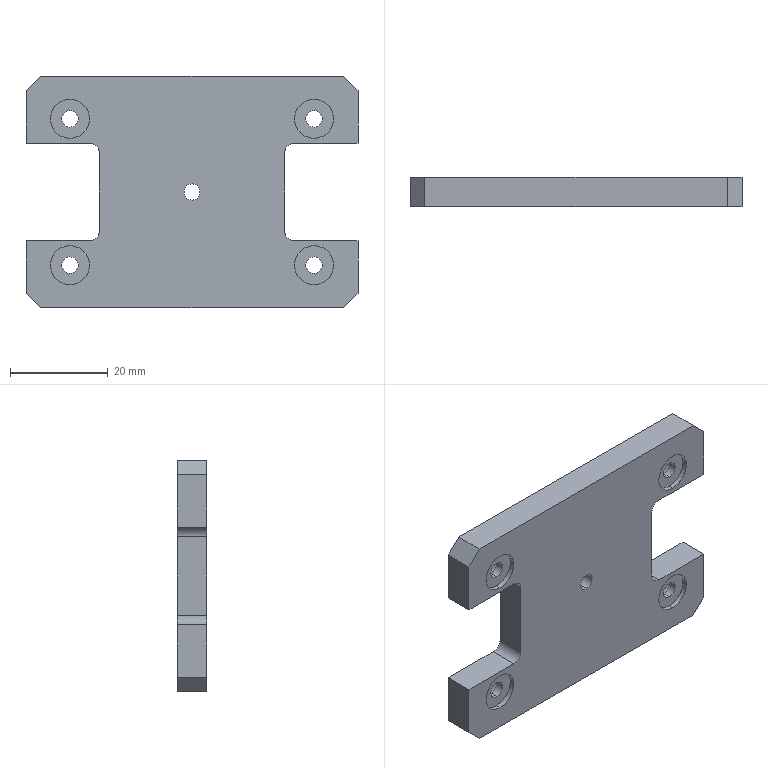Part | STEP file | PN_0040 | 1 solid | 59 faces | box 68 x 6 x 47.5 mm | volume 14110 mm3 | cylinder 32 | plane 27 | commonest cylinder face diameters 3.4 x8 6.5 x8 8 x8 4 x4 3.3 x2 32.5 x2